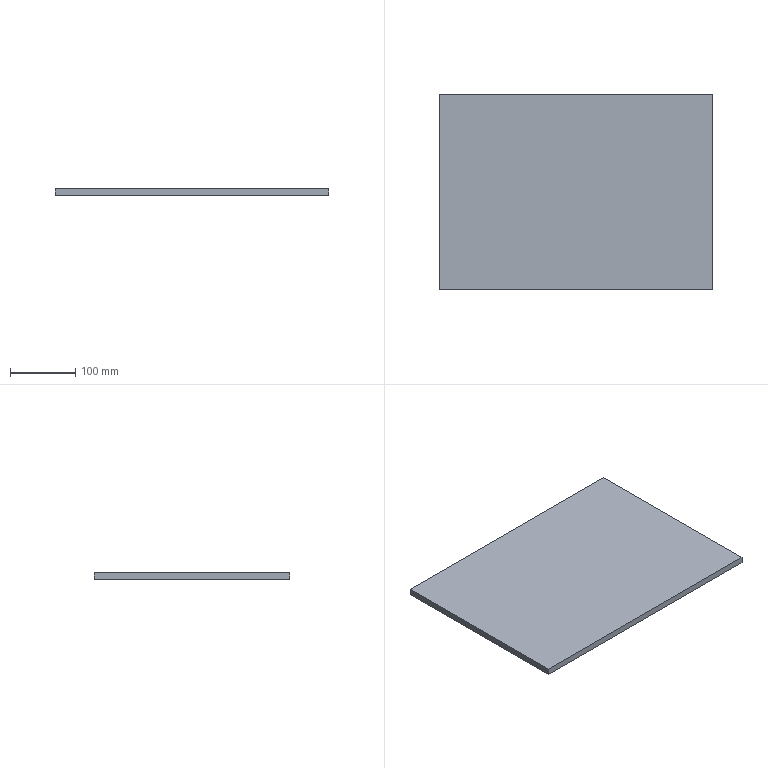Part | STEP file | MYT-A01-P35 | 1 solid | 6 faces | box 420 x 300 x 10 mm | volume 1260000 mm3 | plane 6
STEP:
#1=CARTESIAN_POINT('',(210.,-150.,0.));
#2=VERTEX_POINT('',#1);
#3=CARTESIAN_POINT('',(210.,150.,0.));
#4=VERTEX_POINT('',#3);
#5=CARTESIAN_POINT('',(210.,150.,0.));
#6=DIRECTION('',(0.,1.,0.));
#7=VECTOR('',#6,1000.);
#8=LINE('',#5,#7);
#9=EDGE_CURVE('',#2,#4,#8,.T.);
#10=ORIENTED_EDGE('',*,*,#9,.T.);
#11=CARTESIAN_POINT('',(210.,150.,10.));
#12=VERTEX_POINT('',#11);
#13=CARTESIAN_POINT('',(210.,150.,10.));
#14=DIRECTION('',(0.,0.,-1.));
#15=VECTOR('',#14,1000.);
#16=LINE('',#13,#15);
#17=EDGE_CURVE('',#12,#4,#16,.T.);
#18=ORIENTED_EDGE('',*,*,#17,.F.);
#19=CARTESIAN_POINT('',(210.,-150.,10.));
#20=VERTEX_POINT('',#19);
#21=CARTESIAN_POINT('',(210.,150.,10.));
#22=DIRECTION('',(0.,1.,0.));
#23=VECTOR('',#22,1000.);
#24=LINE('',#21,#23);
#25=EDGE_CURVE('',#20,#12,#24,.T.);
#26=ORIENTED_EDGE('',*,*,#25,.F.);
#27=CARTESIAN_POINT('',(210.,-150.,10.));
#28=DIRECTION('',(0.,0.,-1.));
#29=VECTOR('',#28,1000.);
#30=LINE('',#27,#29);
#31=EDGE_CURVE('',#20,#2,#30,.T.);
#32=ORIENTED_EDGE('',*,*,#31,.T.);
#33=EDGE_LOOP('',(#10,#18,#26,#32));
#34=FACE_OUTER_BOUND('',#33,.T.);
#35=CARTESIAN_POINT('',(210.,150.,10.));
#36=DIRECTION('',(-1.,0.,0.));
#37=DIRECTION('',(0.,-1.,0.));
#38=AXIS2_PLACEMENT_3D('',#35,#36,#37);
#39=PLANE('',#38);
#40=ADVANCED_FACE('',(#34),#39,.F.);
#41=CARTESIAN_POINT('',(-210.,150.,0.));
#42=VERTEX_POINT('',#41);
#43=CARTESIAN_POINT('',(-210.,150.,0.));
#44=DIRECTION('',(-1.,0.,0.));
#45=VECTOR('',#44,1000.);
#46=LINE('',#43,#45);
#47=EDGE_CURVE('',#4,#42,#46,.T.);
#48=ORIENTED_EDGE('',*,*,#47,.T.);
#49=CARTESIAN_POINT('',(-210.,150.,10.));
#50=VERTEX_POINT('',#49);
#51=CARTESIAN_POINT('',(-210.,150.,10.));
#52=DIRECTION('',(0.,0.,-1.));
#53=VECTOR('',#52,1000.);
#54=LINE('',#51,#53);
#55=EDGE_CURVE('',#50,#42,#54,.T.);
#56=ORIENTED_EDGE('',*,*,#55,.F.);
#57=CARTESIAN_POINT('',(-210.,150.,10.));
#58=DIRECTION('',(-1.,0.,0.));
#59=VECTOR('',#58,1000.);
#60=LINE('',#57,#59);
#61=EDGE_CURVE('',#12,#50,#60,.T.);
#62=ORIENTED_EDGE('',*,*,#61,.F.);
#63=ORIENTED_EDGE('',*,*,#17,.T.);
#64=EDGE_LOOP('',(#48,#56,#62,#63));
#65=FACE_OUTER_BOUND('',#64,.T.);
#66=CARTESIAN_POINT('',(-210.,150.,10.));
#67=DIRECTION('',(0.,-1.,0.));
#68=DIRECTION('',(0.,0.,-1.));
#69=AXIS2_PLACEMENT_3D('',#66,#67,#68);
#70=PLANE('',#69);
#71=ADVANCED_FACE('',(#65),#70,.F.);
#72=CARTESIAN_POINT('',(-210.,-150.,0.));
#73=VERTEX_POINT('',#72);
#74=CARTESIAN_POINT('',(-210.,150.,0.));
#75=DIRECTION('',(0.,-1.,0.));
#76=VECTOR('',#75,1000.);
#77=LINE('',#74,#76);
#78=EDGE_CURVE('',#42,#73,#77,.T.);
#79=ORIENTED_EDGE('',*,*,#78,.T.);
#80=CARTESIAN_POINT('',(-210.,-150.,10.));
#81=VERTEX_POINT('',#80);
#82=CARTESIAN_POINT('',(-210.,-150.,10.));
#83=DIRECTION('',(0.,0.,-1.));
#84=VECTOR('',#83,1000.);
#85=LINE('',#82,#84);
#86=EDGE_CURVE('',#81,#73,#85,.T.);
#87=ORIENTED_EDGE('',*,*,#86,.F.);
#88=CARTESIAN_POINT('',(-210.,150.,10.));
#89=DIRECTION('',(0.,-1.,0.));
#90=VECTOR('',#89,1000.);
#91=LINE('',#88,#90);
#92=EDGE_CURVE('',#50,#81,#91,.T.);
#93=ORIENTED_EDGE('',*,*,#92,.F.);
#94=ORIENTED_EDGE('',*,*,#55,.T.);
#95=EDGE_LOOP('',(#79,#87,#93,#94));
#96=FACE_OUTER_BOUND('',#95,.T.);
#97=CARTESIAN_POINT('',(-210.,150.,10.));
#98=DIRECTION('',(1.,0.,0.));
#99=DIRECTION('',(0.,1.,0.));
#100=AXIS2_PLACEMENT_3D('',#97,#98,#99);
#101=PLANE('',#100);
#102=ADVANCED_FACE('',(#96),#101,.F.);
#103=CARTESIAN_POINT('',(-210.,-150.,0.));
#104=DIRECTION('',(1.,0.,0.));
#105=VECTOR('',#104,1000.);
#106=LINE('',#103,#105);
#107=EDGE_CURVE('',#73,#2,#106,.T.);
#108=ORIENTED_EDGE('',*,*,#107,.T.);
#109=ORIENTED_EDGE('',*,*,#31,.F.);
#110=CARTESIAN_POINT('',(-210.,-150.,10.));
#111=DIRECTION('',(1.,0.,0.));
#112=VECTOR('',#111,1000.);
#113=LINE('',#110,#112);
#114=EDGE_CURVE('',#81,#20,#113,.T.);
#115=ORIENTED_EDGE('',*,*,#114,.F.);
#116=ORIENTED_EDGE('',*,*,#86,.T.);
#117=EDGE_LOOP('',(#108,#109,#115,#116));
#118=FACE_OUTER_BOUND('',#117,.T.);
#119=CARTESIAN_POINT('',(-210.,-150.,10.));
#120=DIRECTION('',(0.,1.,0.));
#121=DIRECTION('',(0.,0.,1.));
#122=AXIS2_PLACEMENT_3D('',#119,#120,#121);
#123=PLANE('',#122);
#124=ADVANCED_FACE('',(#118),#123,.F.);
#125=ORIENTED_EDGE('',*,*,#25,.T.);
#126=ORIENTED_EDGE('',*,*,#61,.T.);
#127=ORIENTED_EDGE('',*,*,#92,.T.);
#128=ORIENTED_EDGE('',*,*,#114,.T.);
#129=EDGE_LOOP('',(#125,#126,#127,#128));
#130=FACE_OUTER_BOUND('',#129,.T.);
#131=CARTESIAN_POINT('',(0.,0.,10.));
#132=DIRECTION('',(0.,0.,1.));
#133=DIRECTION('',(1.,0.,0.));
#134=AXIS2_PLACEMENT_3D('',#131,#132,#133);
#135=PLANE('',#134);
#136=ADVANCED_FACE('',(#130),#135,.T.);
#137=ORIENTED_EDGE('',*,*,#9,.F.);
#138=ORIENTED_EDGE('',*,*,#107,.F.);
#139=ORIENTED_EDGE('',*,*,#78,.F.);
#140=ORIENTED_EDGE('',*,*,#47,.F.);
#141=EDGE_LOOP('',(#137,#138,#139,#140));
#142=FACE_OUTER_BOUND('',#141,.T.);
#143=CARTESIAN_POINT('',(0.,0.,0.));
#144=DIRECTION('',(0.,0.,1.));
#145=DIRECTION('',(1.,0.,0.));
#146=AXIS2_PLACEMENT_3D('',#143,#144,#145);
#147=PLANE('',#146);
#148=ADVANCED_FACE('',(#142),#147,.F.);
#149=CLOSED_SHELL('',(#40,#71,#102,#124,#136,#148));
#150=MANIFOLD_SOLID_BREP('',#149);
#151=CARTESIAN_POINT('',(0.,0.,0.));
#152=DIRECTION('',(0.,0.,1.));
#153=DIRECTION('',(1.,0.,0.));
#154=AXIS2_PLACEMENT_3D('',#151,#152,#153);
#155=(LENGTH_UNIT()NAMED_UNIT(*)SI_UNIT(.MILLI.,.METRE.));
#156=UNCERTAINTY_MEASURE_WITH_UNIT(LENGTH_MEASURE(0.00001),#155,'','');
#157=(NAMED_UNIT(*)PLANE_ANGLE_UNIT()SI_UNIT($,.RADIAN.));
#158=(NAMED_UNIT(*)SI_UNIT($,.STERADIAN.)SOLID_ANGLE_UNIT());
#159=(GEOMETRIC_REPRESENTATION_CONTEXT(3)GLOBAL_UNCERTAINTY_ASSIGNED_CONTEXT((#156))GLOBAL_UNIT_ASSIGNED_CONTEXT((#155,#157,#158))REPRESENTATION_CONTEXT('',''));
#160=ADVANCED_BREP_SHAPE_REPRESENTATION('',(#150,#154),#159);